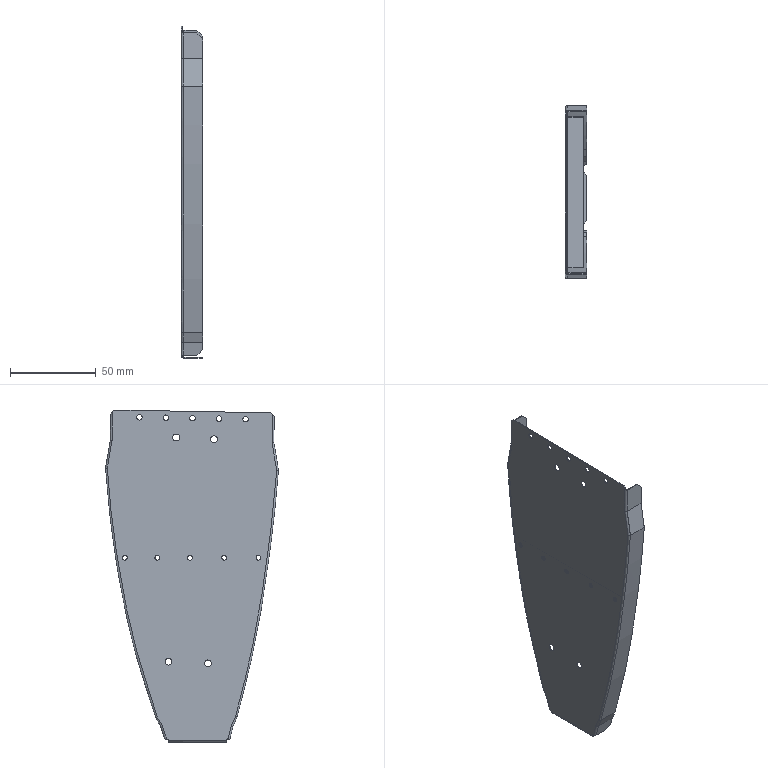Part | SolidWorks | features BaseBody 2 | 2 solids | 126 faces | box 12.5 x 100.931 x 193.879 mm | volume 10991 mm3 | cylinder 66 | plane 50 | spline 9 | cone 1 | commonest cylinder face diameters 2 x21 2.807 x20 3.2 x14 4 x8 1 x1 1.933 x1